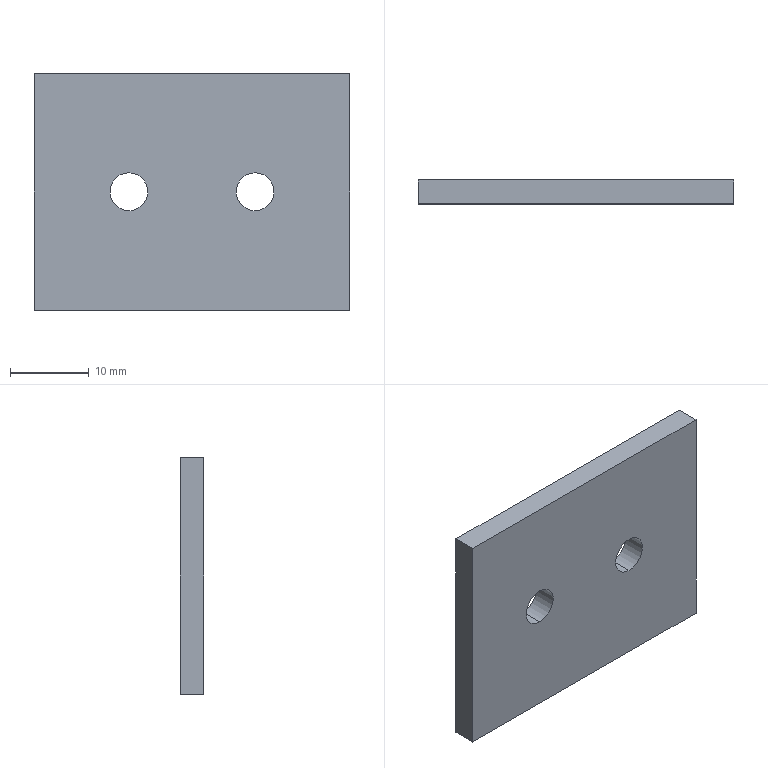Part | SolidWorks | features 3DProfileFeature 1, Extrusion 1, HoleWzd 1 | 1 solid | 10 faces | box 40 x 3 x 30 mm | volume 3491 mm3 | plane 6 | cylinder 4 | commonest cylinder face diameters 4.8 x4
STEP:
#1=CARTESIAN_POINT('',(-8.,3.,-2.369));
#2=VERTEX_POINT('',#1);
#3=CARTESIAN_POINT('',(-8.,3.,2.431));
#4=VERTEX_POINT('',#3);
#5=CARTESIAN_POINT('',(-8.,3.,0.0309));
#6=DIRECTION('',(0.,1.,0.));
#7=DIRECTION('',(0.,0.,1.));
#8=AXIS2_PLACEMENT_3D('',#5,#6,#7);
#9=CIRCLE('',#8,2.4);
#10=EDGE_CURVE('',#2,#4,#9,.T.);
#11=ORIENTED_EDGE('',*,*,#10,.T.);
#12=CARTESIAN_POINT('',(-8.,0.,2.431));
#13=VERTEX_POINT('',#12);
#14=CARTESIAN_POINT('',(-8.,0.,2.431));
#15=DIRECTION('',(0.,-1.,0.));
#16=VECTOR('',#15,1000.);
#17=LINE('',#14,#16);
#18=EDGE_CURVE('',#4,#13,#17,.T.);
#19=ORIENTED_EDGE('',*,*,#18,.T.);
#20=CARTESIAN_POINT('',(-8.,0.,-2.369));
#21=VERTEX_POINT('',#20);
#22=CARTESIAN_POINT('',(-8.,0.,0.0309));
#23=DIRECTION('',(0.,-1.,0.));
#24=DIRECTION('',(0.,0.,-1.));
#25=AXIS2_PLACEMENT_3D('',#22,#23,#24);
#26=CIRCLE('',#25,2.4);
#27=EDGE_CURVE('',#13,#21,#26,.T.);
#28=ORIENTED_EDGE('',*,*,#27,.T.);
#29=CARTESIAN_POINT('',(-8.,0.,-2.369));
#30=DIRECTION('',(0.,-1.,0.));
#31=VECTOR('',#30,1000.);
#32=LINE('',#29,#31);
#33=EDGE_CURVE('',#2,#21,#32,.T.);
#34=ORIENTED_EDGE('',*,*,#33,.F.);
#35=EDGE_LOOP('',(#11,#19,#28,#34));
#36=FACE_OUTER_BOUND('',#35,.T.);
#37=CARTESIAN_POINT('',(-8.,0.,0.0309));
#38=DIRECTION('',(0.,-1.,0.));
#39=DIRECTION('',(0.,0.,-1.));
#40=AXIS2_PLACEMENT_3D('',#37,#38,#39);
#41=CYLINDRICAL_SURFACE('',#40,2.4);
#42=ADVANCED_FACE('',(#36),#41,.F.);
#43=CARTESIAN_POINT('',(8.,3.,-2.369));
#44=VERTEX_POINT('',#43);
#45=CARTESIAN_POINT('',(8.,3.,2.431));
#46=VERTEX_POINT('',#45);
#47=CARTESIAN_POINT('',(8.,3.,0.0309));
#48=DIRECTION('',(0.,1.,0.));
#49=DIRECTION('',(0.,0.,1.));
#50=AXIS2_PLACEMENT_3D('',#47,#48,#49);
#51=CIRCLE('',#50,2.4);
#52=EDGE_CURVE('',#44,#46,#51,.T.);
#53=ORIENTED_EDGE('',*,*,#52,.T.);
#54=CARTESIAN_POINT('',(8.,0.,2.431));
#55=VERTEX_POINT('',#54);
#56=CARTESIAN_POINT('',(8.,0.,2.431));
#57=DIRECTION('',(0.,-1.,0.));
#58=VECTOR('',#57,1000.);
#59=LINE('',#56,#58);
#60=EDGE_CURVE('',#46,#55,#59,.T.);
#61=ORIENTED_EDGE('',*,*,#60,.T.);
#62=CARTESIAN_POINT('',(8.,0.,-2.369));
#63=VERTEX_POINT('',#62);
#64=CARTESIAN_POINT('',(8.,0.,0.0309));
#65=DIRECTION('',(0.,-1.,0.));
#66=DIRECTION('',(0.,0.,-1.));
#67=AXIS2_PLACEMENT_3D('',#64,#65,#66);
#68=CIRCLE('',#67,2.4);
#69=EDGE_CURVE('',#55,#63,#68,.T.);
#70=ORIENTED_EDGE('',*,*,#69,.T.);
#71=CARTESIAN_POINT('',(8.,0.,-2.369));
#72=DIRECTION('',(0.,-1.,0.));
#73=VECTOR('',#72,1000.);
#74=LINE('',#71,#73);
#75=EDGE_CURVE('',#44,#63,#74,.T.);
#76=ORIENTED_EDGE('',*,*,#75,.F.);
#77=EDGE_LOOP('',(#53,#61,#70,#76));
#78=FACE_OUTER_BOUND('',#77,.T.);
#79=CARTESIAN_POINT('',(8.,0.,0.0309));
#80=DIRECTION('',(0.,-1.,0.));
#81=DIRECTION('',(0.,0.,-1.));
#82=AXIS2_PLACEMENT_3D('',#79,#80,#81);
#83=CYLINDRICAL_SURFACE('',#82,2.4);
#84=ADVANCED_FACE('',(#78),#83,.F.);
#85=CARTESIAN_POINT('',(8.,0.,0.0309));
#86=DIRECTION('',(0.,-1.,0.));
#87=DIRECTION('',(0.,0.,-1.));
#88=AXIS2_PLACEMENT_3D('',#85,#86,#87);
#89=CIRCLE('',#88,2.4);
#90=EDGE_CURVE('',#63,#55,#89,.T.);
#91=ORIENTED_EDGE('',*,*,#90,.F.);
#92=ORIENTED_EDGE('',*,*,#69,.F.);
#93=EDGE_LOOP('',(#91,#92));
#94=FACE_BOUND('',#93,.T.);
#95=CARTESIAN_POINT('',(20.,0.,15.));
#96=VERTEX_POINT('',#95);
#97=CARTESIAN_POINT('',(20.,0.,-15.));
#98=VERTEX_POINT('',#97);
#99=CARTESIAN_POINT('',(20.,0.,-15.));
#100=DIRECTION('',(0.,0.,-1.));
#101=VECTOR('',#100,1000.);
#102=LINE('',#99,#101);
#103=EDGE_CURVE('',#96,#98,#102,.T.);
#104=ORIENTED_EDGE('',*,*,#103,.F.);
#105=CARTESIAN_POINT('',(-20.,0.,15.));
#106=VERTEX_POINT('',#105);
#107=CARTESIAN_POINT('',(-20.,0.,15.));
#108=DIRECTION('',(1.,0.,0.));
#109=VECTOR('',#108,1000.);
#110=LINE('',#107,#109);
#111=EDGE_CURVE('',#106,#96,#110,.T.);
#112=ORIENTED_EDGE('',*,*,#111,.F.);
#113=CARTESIAN_POINT('',(-20.,0.,-15.));
#114=VERTEX_POINT('',#113);
#115=CARTESIAN_POINT('',(-20.,0.,-15.));
#116=DIRECTION('',(0.,0.,1.));
#117=VECTOR('',#116,1000.);
#118=LINE('',#115,#117);
#119=EDGE_CURVE('',#114,#106,#118,.T.);
#120=ORIENTED_EDGE('',*,*,#119,.F.);
#121=CARTESIAN_POINT('',(-20.,0.,-15.));
#122=DIRECTION('',(-1.,0.,0.));
#123=VECTOR('',#122,1000.);
#124=LINE('',#121,#123);
#125=EDGE_CURVE('',#98,#114,#124,.T.);
#126=ORIENTED_EDGE('',*,*,#125,.F.);
#127=EDGE_LOOP('',(#104,#112,#120,#126));
#128=FACE_OUTER_BOUND('',#127,.T.);
#129=CARTESIAN_POINT('',(-8.,0.,0.0309));
#130=DIRECTION('',(0.,-1.,0.));
#131=DIRECTION('',(0.,0.,-1.));
#132=AXIS2_PLACEMENT_3D('',#129,#130,#131);
#133=CIRCLE('',#132,2.4);
#134=EDGE_CURVE('',#21,#13,#133,.T.);
#135=ORIENTED_EDGE('',*,*,#134,.F.);
#136=ORIENTED_EDGE('',*,*,#27,.F.);
#137=EDGE_LOOP('',(#135,#136));
#138=FACE_BOUND('',#137,.T.);
#139=CARTESIAN_POINT('',(0.,0.,0.));
#140=DIRECTION('',(0.,1.,0.));
#141=DIRECTION('',(0.,0.,1.));
#142=AXIS2_PLACEMENT_3D('',#139,#140,#141);
#143=PLANE('',#142);
#144=ADVANCED_FACE('',(#94,#128,#138),#143,.F.);
#145=ORIENTED_EDGE('',*,*,#103,.T.);
#146=CARTESIAN_POINT('',(20.,3.,-15.));
#147=VERTEX_POINT('',#146);
#148=CARTESIAN_POINT('',(20.,3.,-15.));
#149=DIRECTION('',(0.,-1.,0.));
#150=VECTOR('',#149,1000.);
#151=LINE('',#148,#150);
#152=EDGE_CURVE('',#147,#98,#151,.T.);
#153=ORIENTED_EDGE('',*,*,#152,.F.);
#154=CARTESIAN_POINT('',(20.,3.,15.));
#155=VERTEX_POINT('',#154);
#156=CARTESIAN_POINT('',(20.,3.,-15.));
#157=DIRECTION('',(0.,0.,-1.));
#158=VECTOR('',#157,1000.);
#159=LINE('',#156,#158);
#160=EDGE_CURVE('',#155,#147,#159,.T.);
#161=ORIENTED_EDGE('',*,*,#160,.F.);
#162=CARTESIAN_POINT('',(20.,3.,15.));
#163=DIRECTION('',(0.,-1.,0.));
#164=VECTOR('',#163,1000.);
#165=LINE('',#162,#164);
#166=EDGE_CURVE('',#155,#96,#165,.T.);
#167=ORIENTED_EDGE('',*,*,#166,.T.);
#168=EDGE_LOOP('',(#145,#153,#161,#167));
#169=FACE_OUTER_BOUND('',#168,.T.);
#170=CARTESIAN_POINT('',(20.,3.,-15.));
#171=DIRECTION('',(-1.,0.,0.));
#172=DIRECTION('',(0.,0.,1.));
#173=AXIS2_PLACEMENT_3D('',#170,#171,#172);
#174=PLANE('',#173);
#175=ADVANCED_FACE('',(#169),#174,.F.);
#176=ORIENTED_EDGE('',*,*,#125,.T.);
#177=CARTESIAN_POINT('',(-20.,3.,-15.));
#178=VERTEX_POINT('',#177);
#179=CARTESIAN_POINT('',(-20.,3.,-15.));
#180=DIRECTION('',(0.,-1.,0.));
#181=VECTOR('',#180,1000.);
#182=LINE('',#179,#181);
#183=EDGE_CURVE('',#178,#114,#182,.T.);
#184=ORIENTED_EDGE('',*,*,#183,.F.);
#185=CARTESIAN_POINT('',(-20.,3.,-15.));
#186=DIRECTION('',(-1.,0.,0.));
#187=VECTOR('',#186,1000.);
#188=LINE('',#185,#187);
#189=EDGE_CURVE('',#147,#178,#188,.T.);
#190=ORIENTED_EDGE('',*,*,#189,.F.);
#191=ORIENTED_EDGE('',*,*,#152,.T.);
#192=EDGE_LOOP('',(#176,#184,#190,#191));
#193=FACE_OUTER_BOUND('',#192,.T.);
#194=CARTESIAN_POINT('',(-20.,3.,-15.));
#195=DIRECTION('',(0.,0.,1.));
#196=DIRECTION('',(1.,0.,0.));
#197=AXIS2_PLACEMENT_3D('',#194,#195,#196);
#198=PLANE('',#197);
#199=ADVANCED_FACE('',(#193),#198,.F.);
#200=ORIENTED_EDGE('',*,*,#119,.T.);
#201=CARTESIAN_POINT('',(-20.,3.,15.));
#202=VERTEX_POINT('',#201);
#203=CARTESIAN_POINT('',(-20.,3.,15.));
#204=DIRECTION('',(0.,-1.,0.));
#205=VECTOR('',#204,1000.);
#206=LINE('',#203,#205);
#207=EDGE_CURVE('',#202,#106,#206,.T.);
#208=ORIENTED_EDGE('',*,*,#207,.F.);
#209=CARTESIAN_POINT('',(-20.,3.,-15.));
#210=DIRECTION('',(0.,0.,1.));
#211=VECTOR('',#210,1000.);
#212=LINE('',#209,#211);
#213=EDGE_CURVE('',#178,#202,#212,.T.);
#214=ORIENTED_EDGE('',*,*,#213,.F.);
#215=ORIENTED_EDGE('',*,*,#183,.T.);
#216=EDGE_LOOP('',(#200,#208,#214,#215));
#217=FACE_OUTER_BOUND('',#216,.T.);
#218=CARTESIAN_POINT('',(-20.,3.,-15.));
#219=DIRECTION('',(1.,0.,0.));
#220=DIRECTION('',(0.,0.,-1.));
#221=AXIS2_PLACEMENT_3D('',#218,#219,#220);
#222=PLANE('',#221);
#223=ADVANCED_FACE('',(#217),#222,.F.);
#224=ORIENTED_EDGE('',*,*,#111,.T.);
#225=ORIENTED_EDGE('',*,*,#166,.F.);
#226=CARTESIAN_POINT('',(-20.,3.,15.));
#227=DIRECTION('',(1.,0.,0.));
#228=VECTOR('',#227,1000.);
#229=LINE('',#226,#228);
#230=EDGE_CURVE('',#202,#155,#229,.T.);
#231=ORIENTED_EDGE('',*,*,#230,.F.);
#232=ORIENTED_EDGE('',*,*,#207,.T.);
#233=EDGE_LOOP('',(#224,#225,#231,#232));
#234=FACE_OUTER_BOUND('',#233,.T.);
#235=CARTESIAN_POINT('',(-20.,3.,15.));
#236=DIRECTION('',(0.,0.,-1.));
#237=DIRECTION('',(-1.,0.,0.));
#238=AXIS2_PLACEMENT_3D('',#235,#236,#237);
#239=PLANE('',#238);
#240=ADVANCED_FACE('',(#234),#239,.F.);
#241=ORIENTED_EDGE('',*,*,#10,.F.);
#242=CARTESIAN_POINT('',(-8.,3.,0.0309));
#243=DIRECTION('',(0.,1.,0.));
#244=DIRECTION('',(0.,0.,1.));
#245=AXIS2_PLACEMENT_3D('',#242,#243,#244);
#246=CIRCLE('',#245,2.4);
#247=EDGE_CURVE('',#4,#2,#246,.T.);
#248=ORIENTED_EDGE('',*,*,#247,.F.);
#249=EDGE_LOOP('',(#241,#248));
#250=FACE_BOUND('',#249,.T.);
#251=ORIENTED_EDGE('',*,*,#52,.F.);
#252=CARTESIAN_POINT('',(8.,3.,0.0309));
#253=DIRECTION('',(0.,1.,0.));
#254=DIRECTION('',(0.,0.,1.));
#255=AXIS2_PLACEMENT_3D('',#252,#253,#254);
#256=CIRCLE('',#255,2.4);
#257=EDGE_CURVE('',#46,#44,#256,.T.);
#258=ORIENTED_EDGE('',*,*,#257,.F.);
#259=EDGE_LOOP('',(#251,#258));
#260=FACE_BOUND('',#259,.T.);
#261=ORIENTED_EDGE('',*,*,#160,.T.);
#262=ORIENTED_EDGE('',*,*,#189,.T.);
#263=ORIENTED_EDGE('',*,*,#213,.T.);
#264=ORIENTED_EDGE('',*,*,#230,.T.);
#265=EDGE_LOOP('',(#261,#262,#263,#264));
#266=FACE_OUTER_BOUND('',#265,.T.);
#267=CARTESIAN_POINT('',(0.,3.,0.));
#268=DIRECTION('',(0.,1.,0.));
#269=DIRECTION('',(0.,0.,1.));
#270=AXIS2_PLACEMENT_3D('',#267,#268,#269);
#271=PLANE('',#270);
#272=ADVANCED_FACE('',(#250,#260,#266),#271,.T.);
#273=ORIENTED_EDGE('',*,*,#60,.F.);
#274=ORIENTED_EDGE('',*,*,#257,.T.);
#275=ORIENTED_EDGE('',*,*,#75,.T.);
#276=ORIENTED_EDGE('',*,*,#90,.T.);
#277=EDGE_LOOP('',(#273,#274,#275,#276));
#278=FACE_OUTER_BOUND('',#277,.T.);
#279=CARTESIAN_POINT('',(8.,0.,0.0309));
#280=DIRECTION('',(0.,-1.,0.));
#281=DIRECTION('',(0.,0.,-1.));
#282=AXIS2_PLACEMENT_3D('',#279,#280,#281);
#283=CYLINDRICAL_SURFACE('',#282,2.4);
#284=ADVANCED_FACE('',(#278),#283,.F.);
#285=ORIENTED_EDGE('',*,*,#18,.F.);
#286=ORIENTED_EDGE('',*,*,#247,.T.);
#287=ORIENTED_EDGE('',*,*,#33,.T.);
#288=ORIENTED_EDGE('',*,*,#134,.T.);
#289=EDGE_LOOP('',(#285,#286,#287,#288));
#290=FACE_OUTER_BOUND('',#289,.T.);
#291=CARTESIAN_POINT('',(-8.,0.,0.0309));
#292=DIRECTION('',(0.,-1.,0.));
#293=DIRECTION('',(0.,0.,-1.));
#294=AXIS2_PLACEMENT_3D('',#291,#292,#293);
#295=CYLINDRICAL_SURFACE('',#294,2.4);
#296=ADVANCED_FACE('',(#290),#295,.F.);
#297=CLOSED_SHELL('',(#42,#84,#144,#175,#199,#223,#240,#272,#284,#296));
#298=MANIFOLD_SOLID_BREP('',#297);
#299=CARTESIAN_POINT('',(0.,0.,0.));
#300=DIRECTION('',(0.,0.,1.));
#301=DIRECTION('',(1.,0.,0.));
#302=AXIS2_PLACEMENT_3D('',#299,#300,#301);
#303=(LENGTH_UNIT()NAMED_UNIT(*)SI_UNIT(.MILLI.,.METRE.));
#304=UNCERTAINTY_MEASURE_WITH_UNIT(LENGTH_MEASURE(0.00001),#303,'','');
#305=(NAMED_UNIT(*)PLANE_ANGLE_UNIT()SI_UNIT($,.RADIAN.));
#306=(NAMED_UNIT(*)SI_UNIT($,.STERADIAN.)SOLID_ANGLE_UNIT());
#307=(GEOMETRIC_REPRESENTATION_CONTEXT(3)GLOBAL_UNCERTAINTY_ASSIGNED_CONTEXT((#304))GLOBAL_UNIT_ASSIGNED_CONTEXT((#303,#305,#306))REPRESENTATION_CONTEXT('',''));
#308=ADVANCED_BREP_SHAPE_REPRESENTATION('',(#298,#302),#307);